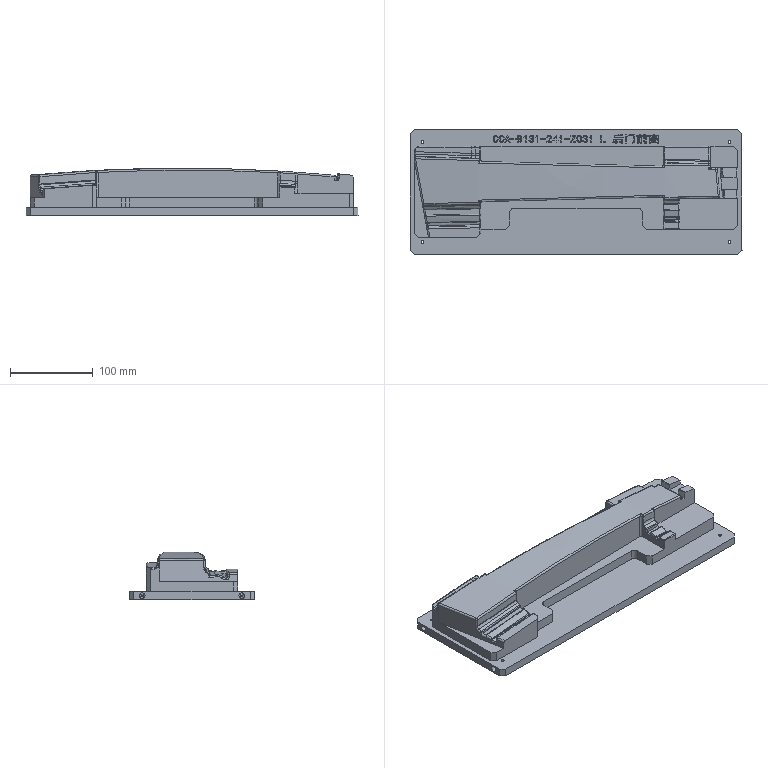NC program | NX | posted with a generic post | part box 400 x 150 x 57.494 mm
Lines 6500 to 7057 of 7057:
(A5 , TOOL : D10)
N12980 M6
N12982 G54
N12984 G17 G0 G90 X-193. Y-85.002 S3500 M3
N12986 G43 Z20.002 H0
N12988 Z9.802
N12990 G94 G1 Z9.502 F2000.
N12992 Y-82.002
N12994 G3 X-195. Y-80.002 R2.
N12996 G2 X-198.536 Y-78.538 R5.
N12998 G1 X-203.536 Y-73.538
N13000 G2 X-205. Y-70.002 R5.
N13002 G1 Y69.998
N13004 G2 X-203.536 Y73.533 R5.
N13006 G1 X-198.536 Y78.533
N13008 G2 X-195. Y79.998 R5.
N13010 G1 X195. Z9.503
N13012 G2 X198.536 Y78.533 R5.
N13014 G1 X203.536 Y73.533
N13016 G2 X205. Y69.998 R5.
N13018 G1 Y-70.002
N13020 G2 X203.536 Y-73.538 R5.
N13022 G1 X198.536 Y-78.538
N13024 G2 X195. Y-80.002 R5.
N13026 G1 X-195. Z9.502
N13028 G3 X-197. Y-82.002 R2.
N13030 G1 Y-84.8
N13032 Z9.802
N13034 G0 Z10.302
N13036 X-193. Y-85.002
N13038 Z9.302
N13040 G1 Z9.002
N13042 Y-82.002
N13044 G3 X-195. Y-80.002 R2.
N13046 G2 X-198.536 Y-78.538 R5.
N13048 G1 X-203.536 Y-73.538
N13050 G2 X-205. Y-70.002 R5.
N13052 G1 Y69.998
N13054 G2 X-203.536 Y73.533 R5.
N13056 G1 X-198.536 Y78.533
N13058 G2 X-195. Y79.998 R5.
N13060 G1 X195. Z9.003
N13062 G2 X198.536 Y78.533 R5.
N13064 G1 X203.536 Y73.533
N13066 G2 X205. Y69.998 R5.
N13068 G1 Y-70.002
N13070 G2 X203.536 Y-73.538 R5.
N13072 G1 X198.536 Y-78.538
N13074 G2 X195. Y-80.002 R5.
N13076 G1 X-195. Z9.002
N13078 G3 X-197. Y-82.002 R2.
N13080 G1 Y-84.8
N13082 Z9.302
N13084 G0 Z9.802
N13086 X-193. Y-85.002
N13088 Z8.802
N13090 G1 Z8.502
N13092 Y-82.002
N13094 G3 X-195. Y-80.002 R2.
N13096 G2 X-198.536 Y-78.538 R5.
N13098 G1 X-203.536 Y-73.538
N13100 G2 X-205. Y-70.002 R5.
N13102 G1 Y69.998
N13104 G2 X-203.536 Y73.533 R5.
N13106 G1 X-198.536 Y78.533
N13108 G2 X-195. Y79.998 R5.
N13110 G1 X195. Z8.503
N13112 G2 X198.536 Y78.533 R5.
N13114 G1 X203.536 Y73.533
N13116 G2 X205. Y69.998 R5.
N13118 G1 Y-70.002
N13120 G2 X203.536 Y-73.538 R5.
N13122 G1 X198.536 Y-78.538
N13124 G2 X195. Y-80.002 R5.
N13126 G1 X-195. Z8.502
N13128 G3 X-197. Y-82.002 R2.
N13130 G1 Y-84.8
N13132 Z8.802
N13134 G0 Z9.302
N13136 X-193. Y-85.002
N13138 Z8.302
N13140 G1 Z8.002
N13142 Y-82.002
N13144 G3 X-195. Y-80.002 R2.
N13146 G2 X-198.536 Y-78.538 R5.
N13148 G1 X-203.536 Y-73.538
N13150 G2 X-205. Y-70.002 R5.
N13152 G1 Y69.998
N13154 G2 X-203.536 Y73.533 R5.
N13156 G1 X-198.536 Y78.533
N13158 G2 X-195. Y79.998 R5.
N13160 G1 X195. Z8.003
N13162 G2 X198.536 Y78.533 R5.
N13164 G1 X203.536 Y73.533
N13166 G2 X205. Y69.998 R5.
N13168 G1 Y-70.002
N13170 G2 X203.536 Y-73.538 R5.
N13172 G1 X198.536 Y-78.538
N13174 G2 X195. Y-80.002 R5.
N13176 G1 X-195. Z8.002
N13178 G3 X-197. Y-82.002 R2.
N13180 G1 Y-84.8
N13182 Z8.302
N13184 G0 Z8.802
N13186 X-193. Y-85.002
N13188 Z7.802
N13190 G1 Z7.502
N13192 Y-82.002
N13194 G3 X-195. Y-80.002 R2.
N13196 G2 X-198.536 Y-78.538 R5.
N13198 G1 X-203.536 Y-73.538
N13200 G2 X-205. Y-70.002 R5.
N13202 G1 Y69.998
N13204 G2 X-203.536 Y73.533 R5.
N13206 G1 X-198.536 Y78.533
N13208 G2 X-195. Y79.998 R5.
N13210 G1 X195. Z7.503
N13212 G2 X198.536 Y78.533 R5.
N13214 G1 X203.536 Y73.533
N13216 G2 X205. Y69.998 R5.
N13218 G1 Y-70.002
N13220 G2 X203.536 Y-73.538 R5.
N13222 G1 X198.536 Y-78.538
N13224 G2 X195. Y-80.002 R5.
N13226 G1 X-195. Z7.502
N13228 G3 X-197. Y-82.002 R2.
N13230 G1 Y-84.8
N13232 Z7.802
N13234 G0 Z8.302
N13236 X-193. Y-85.002
N13238 Z7.302
N13240 G1 Z7.002
N13242 Y-82.002
N13244 G3 X-195. Y-80.002 R2.
N13246 G2 X-198.536 Y-78.538 R5.
N13248 G1 X-203.536 Y-73.538
N13250 G2 X-205. Y-70.002 R5.
N13252 G1 Y69.998
N13254 G2 X-203.536 Y73.533 R5.
N13256 G1 X-198.536 Y78.533
N13258 G2 X-195. Y79.998 R5.
N13260 G1 X195. Z7.003
N13262 G2 X198.536 Y78.533 R5.
N13264 G1 X203.536 Y73.533
N13266 G2 X205. Y69.998 R5.
N13268 G1 Y-70.002
N13270 G2 X203.536 Y-73.538 R5.
N13272 G1 X198.536 Y-78.538
N13274 G2 X195. Y-80.002 R5.
N13276 G1 X-195. Z7.002
N13278 G3 X-197. Y-82.002 R2.
N13280 G1 Y-84.8
N13282 Z7.302
N13284 G0 Z7.802
N13286 X-193. Y-85.002
N13288 Z6.802
N13290 G1 Z6.502
N13292 Y-82.002
N13294 G3 X-195. Y-80.002 R2.
N13296 G2 X-198.536 Y-78.538 R5.
N13298 G1 X-203.536 Y-73.538
N13300 G2 X-205. Y-70.002 R5.
N13302 G1 Y69.998
N13304 G2 X-203.536 Y73.533 R5.
N13306 G1 X-198.536 Y78.533
N13308 G2 X-195. Y79.998 R5.
N13310 G1 X195. Z6.503
N13312 G2 X198.536 Y78.533 R5.
N13314 G1 X203.536 Y73.533
N13316 G2 X205. Y69.998 R5.
N13318 G1 Y-70.002
N13320 G2 X203.536 Y-73.538 R5.
N13322 G1 X198.536 Y-78.538
N13324 G2 X195. Y-80.002 R5.
N13326 G1 X-195. Z6.502
N13328 G3 X-197. Y-82.002 R2.
N13330 G1 Y-84.8
N13332 Z6.802
N13334 G0 Z7.302
N13336 X-193. Y-85.002
N13338 Z6.302
N13340 G1 Z6.002
N13342 Y-82.002
N13344 G3 X-195. Y-80.002 R2.
N13346 G2 X-198.536 Y-78.538 R5.
N13348 G1 X-203.536 Y-73.538
N13350 G2 X-205. Y-70.002 R5.
N13352 G1 Y69.998
N13354 G2 X-203.536 Y73.533 R5.
N13356 G1 X-198.536 Y78.533
N13358 G2 X-195. Y79.998 R5.
N13360 G1 X195. Z6.003
N13362 G2 X198.536 Y78.533 R5.
N13364 G1 X203.536 Y73.533
N13366 G2 X205. Y69.998 R5.
N13368 G1 Y-70.002
N13370 G2 X203.536 Y-73.538 R5.
N13372 G1 X198.536 Y-78.538
N13374 G2 X195. Y-80.002 R5.
N13376 G1 X-195. Z6.002
N13378 G3 X-197. Y-82.002 R2.
N13380 G1 Y-84.8
N13382 Z6.302
N13384 G0 Z6.802
N13386 X-193. Y-85.002
N13388 Z5.802
N13390 G1 Z5.502
N13392 Y-82.002
N13394 G3 X-195. Y-80.002 R2.
N13396 G2 X-198.536 Y-78.538 R5.
N13398 G1 X-203.536 Y-73.538
N13400 G2 X-205. Y-70.002 R5.
N13402 G1 Y69.998
N13404 G2 X-203.536 Y73.533 R5.
N13406 G1 X-198.536 Y78.533
N13408 G2 X-195. Y79.998 R5.
N13410 G1 X195. Z5.503
N13412 G2 X198.536 Y78.533 R5.
N13414 G1 X203.536 Y73.533
N13416 G2 X205. Y69.998 R5.
N13418 G1 Y-70.002
N13420 G2 X203.536 Y-73.538 R5.
N13422 G1 X198.536 Y-78.538
N13424 G2 X195. Y-80.002 R5.
N13426 G1 X-195. Z5.502
N13428 G3 X-197. Y-82.002 R2.
N13430 G1 Y-84.8
N13432 Z5.802
N13434 G0 Z6.302
N13436 X-193. Y-85.002
N13438 Z5.302
N13440 G1 Z5.002
N13442 Y-82.002
N13444 G3 X-195. Y-80.002 R2.
N13446 G2 X-198.536 Y-78.538 R5.
N13448 G1 X-203.536 Y-73.538
N13450 G2 X-205. Y-70.002 R5.
N13452 G1 Y69.998
N13454 G2 X-203.536 Y73.533 R5.
N13456 G1 X-198.536 Y78.533
N13458 G2 X-195. Y79.998 R5.
N13460 G1 X195. Z5.003
N13462 G2 X198.536 Y78.533 R5.
N13464 G1 X203.536 Y73.533
N13466 G2 X205. Y69.998 R5.
N13468 G1 Y-70.002
N13470 G2 X203.536 Y-73.538 R5.
N13472 G1 X198.536 Y-78.538
N13474 G2 X195. Y-80.002 R5.
N13476 G1 X-195. Z5.002
N13478 G3 X-197. Y-82.002 R2.
N13480 G1 Y-84.8
N13482 Z5.302
N13484 G0 Z5.802
N13486 X-193. Y-85.002
N13488 Z4.802
N13490 G1 Z4.502
N13492 Y-82.002
N13494 G3 X-195. Y-80.002 R2.
N13496 G2 X-198.536 Y-78.538 R5.
N13498 G1 X-203.536 Y-73.538
N13500 G2 X-205. Y-70.002 R5.
N13502 G1 Y69.998
N13504 G2 X-203.536 Y73.533 R5.
N13506 G1 X-198.536 Y78.533
N13508 G2 X-195. Y79.998 R5.
N13510 G1 X195. Z4.503
N13512 G2 X198.536 Y78.533 R5.
N13514 G1 X203.536 Y73.533
N13516 G2 X205. Y69.998 R5.
N13518 G1 Y-70.002
N13520 G2 X203.536 Y-73.538 R5.
N13522 G1 X198.536 Y-78.538
N13524 G2 X195. Y-80.002 R5.
N13526 G1 X-195. Z4.502
N13528 G3 X-197. Y-82.002 R2.
N13530 G1 Y-84.8
N13532 Z4.802
N13534 G0 Z5.302
N13536 X-193. Y-85.002
N13538 Z4.302
N13540 G1 Z4.002
N13542 Y-82.002
N13544 G3 X-195. Y-80.002 R2.
N13546 G2 X-198.536 Y-78.538 R5.
N13548 G1 X-203.536 Y-73.538
N13550 G2 X-205. Y-70.002 R5.
N13552 G1 Y69.998
N13554 G2 X-203.536 Y73.533 R5.
N13556 G1 X-198.536 Y78.533
N13558 G2 X-195. Y79.998 R5.
N13560 G1 X195. Z4.003
N13562 G2 X198.536 Y78.533 R5.
N13564 G1 X203.536 Y73.533
N13566 G2 X205. Y69.998 R5.
N13568 G1 Y-70.002
N13570 G2 X203.536 Y-73.538 R5.
N13572 G1 X198.536 Y-78.538
N13574 G2 X195. Y-80.002 R5.
N13576 G1 X-195. Z4.002
N13578 G3 X-197. Y-82.002 R2.
N13580 G1 Y-84.8
N13582 Z4.302
N13584 G0 Z4.802
N13586 X-193. Y-85.002
N13588 Z3.802
N13590 G1 Z3.502
N13592 Y-82.002
N13594 G3 X-195. Y-80.002 R2.
N13596 G2 X-198.536 Y-78.538 R5.
N13598 G1 X-203.536 Y-73.538
N13600 G2 X-205. Y-70.002 R5.
N13602 G1 Y69.998
N13604 G2 X-203.536 Y73.533 R5.
N13606 G1 X-198.536 Y78.533
N13608 G2 X-195. Y79.998 R5.
N13610 G1 X195. Z3.503
N13612 G2 X198.536 Y78.533 R5.
N13614 G1 X203.536 Y73.533
N13616 G2 X205. Y69.998 R5.
N13618 G1 Y-70.002
N13620 G2 X203.536 Y-73.538 R5.
N13622 G1 X198.536 Y-78.538
N13624 G2 X195. Y-80.002 R5.
N13626 G1 X-195. Z3.502
N13628 G3 X-197. Y-82.002 R2.
N13630 G1 Y-84.8
N13632 Z3.802
N13634 G0 Z4.302
N13636 X-193. Y-85.002
N13638 Z3.302
N13640 G1 Z3.002
N13642 Y-82.002
N13644 G3 X-195. Y-80.002 R2.
N13646 G2 X-198.536 Y-78.538 R5.
N13648 G1 X-203.536 Y-73.538
N13650 G2 X-205. Y-70.002 R5.
N13652 G1 Y69.998
N13654 G2 X-203.536 Y73.533 R5.
N13656 G1 X-198.536 Y78.533
N13658 G2 X-195. Y79.998 R5.
N13660 G1 X195. Z3.003
N13662 G2 X198.536 Y78.533 R5.
N13664 G1 X203.536 Y73.533
N13666 G2 X205. Y69.998 R5.
N13668 G1 Y-70.002
N13670 G2 X203.536 Y-73.538 R5.
N13672 G1 X198.536 Y-78.538
N13674 G2 X195. Y-80.002 R5.
N13676 G1 X-195. Z3.002
N13678 G3 X-197. Y-82.002 R2.
N13680 G1 Y-84.8
N13682 Z3.302
N13684 G0 Z3.802
N13686 X-193. Y-85.002
N13688 Z2.802
N13690 G1 Z2.502
N13692 Y-82.002
N13694 G3 X-195. Y-80.002 R2.
N13696 G2 X-198.536 Y-78.538 R5.
N13698 G1 X-203.536 Y-73.538
N13700 G2 X-205. Y-70.002 R5.
N13702 G1 Y69.998
N13704 G2 X-203.536 Y73.533 R5.
N13706 G1 X-198.536 Y78.533
N13708 G2 X-195. Y79.998 R5.
N13710 G1 X195. Z2.503
N13712 G2 X198.536 Y78.533 R5.
N13714 G1 X203.536 Y73.533
N13716 G2 X205. Y69.998 R5.
N13718 G1 Y-70.002
N13720 G2 X203.536 Y-73.538 R5.
N13722 G1 X198.536 Y-78.538
N13724 G2 X195. Y-80.002 R5.
N13726 G1 X-195. Z2.502
N13728 G3 X-197. Y-82.002 R2.
N13730 G1 Y-84.8
N13732 Z2.802
N13734 G0 Z3.302
N13736 X-193. Y-85.002
N13738 Z2.302
N13740 G1 Z2.002
N13742 Y-82.002
N13744 G3 X-195. Y-80.002 R2.
N13746 G2 X-198.536 Y-78.538 R5.
N13748 G1 X-203.536 Y-73.538
N13750 G2 X-205. Y-70.002 R5.
N13752 G1 Y69.998
N13754 G2 X-203.536 Y73.533 R5.
N13756 G1 X-198.536 Y78.533
N13758 G2 X-195. Y79.998 R5.
N13760 G1 X195. Z2.003
N13762 G2 X198.536 Y78.533 R5.
N13764 G1 X203.536 Y73.533
N13766 G2 X205. Y69.998 R5.
N13768 G1 Y-70.002
N13770 G2 X203.536 Y-73.538 R5.
N13772 G1 X198.536 Y-78.538
N13774 G2 X195. Y-80.002 R5.
N13776 G1 X-195. Z2.002
N13778 G3 X-197. Y-82.002 R2.
N13780 G1 Y-84.8
N13782 Z2.302
N13784 G0 Z2.802
N13786 X-193. Y-85.002
N13788 Z1.802
N13790 G1 Z1.502
N13792 Y-82.002
N13794 G3 X-195. Y-80.002 R2.
N13796 G2 X-198.536 Y-78.538 R5.
N13798 G1 X-203.536 Y-73.538
N13800 G2 X-205. Y-70.002 R5.
N13802 G1 Y69.998
N13804 G2 X-203.536 Y73.533 R5.
N13806 G1 X-198.536 Y78.533
N13808 G2 X-195. Y79.998 R5.
N13810 G1 X195. Z1.503
N13812 G2 X198.536 Y78.533 R5.
N13814 G1 X203.536 Y73.533
N13816 G2 X205. Y69.998 R5.
N13818 G1 Y-70.002
N13820 G2 X203.536 Y-73.538 R5.
N13822 G1 X198.536 Y-78.538
N13824 G2 X195. Y-80.002 R5.
N13826 G1 X-195. Z1.502
N13828 G3 X-197. Y-82.002 R2.
N13830 G1 Y-84.8
N13832 Z1.802
N13834 G0 Z2.302
N13836 X-193. Y-85.002
N13838 Z1.302
N13840 G1 Z1.002
N13842 Y-82.002
N13844 G3 X-195. Y-80.002 R2.
N13846 G2 X-198.536 Y-78.538 R5.
N13848 G1 X-203.536 Y-73.538
N13850 G2 X-205. Y-70.002 R5.
N13852 G1 Y69.998
N13854 G2 X-203.536 Y73.533 R5.
N13856 G1 X-198.536 Y78.533
N13858 G2 X-195. Y79.998 R5.
N13860 G1 X195. Z1.003
N13862 G2 X198.536 Y78.533 R5.
N13864 G1 X203.536 Y73.533
N13866 G2 X205. Y69.998 R5.
N13868 G1 Y-70.002
N13870 G2 X203.536 Y-73.538 R5.
N13872 G1 X198.536 Y-78.538
N13874 G2 X195. Y-80.002 R5.
N13876 G1 X-195. Z1.002
N13878 G3 X-197. Y-82.002 R2.
N13880 G1 Y-84.8
N13882 Z1.302
N13884 G0 Z1.802
N13886 X-193. Y-85.002
N13888 Z0.802
N13890 G1 Z0.502
N13892 Y-82.002
N13894 G3 X-195. Y-80.002 R2.
N13896 G2 X-198.536 Y-78.538 R5.
N13898 G1 X-203.536 Y-73.538
N13900 G2 X-205. Y-70.002 R5.
N13902 G1 Y69.998
N13904 G2 X-203.536 Y73.533 R5.
N13906 G1 X-198.536 Y78.533
N13908 G2 X-195. Y79.998 R5.
N13910 G1 X195. Z0.503
N13912 G2 X198.536 Y78.533 R5.
N13914 G1 X203.536 Y73.533
N13916 G2 X205. Y69.998 R5.
N13918 G1 Y-70.002
N13920 G2 X203.536 Y-73.538 R5.
N13922 G1 X198.536 Y-78.538
N13924 G2 X195. Y-80.002 R5.
N13926 G1 X-195. Z0.502
N13928 G3 X-197. Y-82.002 R2.
N13930 G1 Y-84.8
N13932 Z0.802
N13934 G0 Z1.302
N13936 X-193. Y-85.002
N13938 Z0.302
N13940 G1 Z0.002
N13942 Y-82.002
N13944 G3 X-195. Y-80.002 R2.
N13946 G2 X-198.536 Y-78.538 R5.
N13948 G1 X-203.536 Y-73.538
N13950 G2 X-205. Y-70.002 R5.
N13952 G1 Y69.998
N13954 G2 X-203.536 Y73.533 R5.
N13956 G1 X-198.536 Y78.533
N13958 G2 X-195. Y79.998 R5.
N13960 G1 X195. Z0.003
N13962 G2 X198.536 Y78.533 R5.
N13964 G1 X203.536 Y73.533
N13966 G2 X205. Y69.998 R5.
N13968 G1 Y-70.002
N13970 G2 X203.536 Y-73.538 R5.
N13972 G1 X198.536 Y-78.538
N13974 G2 X195. Y-80.002 R5.
N13976 G1 X-195. Z0.002
N13978 G3 X-197. Y-82.002 R2.
N13980 G1 Y-84.8
N13982 Z0.302
N13984 G0 Z0.802
N13986 X-193. Y-85.002
N13988 Z-0.198
N13990 G1 Z-0.498
N13992 Y-82.002
N13994 G3 X-195. Y-80.002 R2.
N13996 G2 X-198.536 Y-78.538 R5.
N13998 G1 X-203.536 Y-73.538
N14000 G2 X-205. Y-70.002 R5.
N14002 G1 Y69.998
N14004 G2 X-203.536 Y73.533 R5.
N14006 G1 X-198.536 Y78.533
N14008 G2 X-195. Y79.998 R5.
N14010 G1 X195. Z-0.497
N14012 G2 X198.536 Y78.533 R5.
N14014 G1 X203.536 Y73.533
N14016 G2 X205. Y69.998 R5.
N14018 G1 Y-70.002
N14020 G2 X203.536 Y-73.538 R5.
N14022 G1 X198.536 Y-78.538
N14024 G2 X195. Y-80.002 R5.
N14026 G1 X-195. Z-0.498
N14028 G3 X-197. Y-82.002 R2.
N14030 G1 Y-84.8
N14032 Z-0.198
N14034 G0 Z0.302
N14036 X-193. Y-85.002
N14038 Z-0.698
N14040 G1 Z-0.998
N14042 Y-82.002
N14044 G3 X-195. Y-80.002 R2.
N14046 G2 X-198.536 Y-78.538 R5.
N14048 G1 X-203.536 Y-73.538
N14050 G2 X-205. Y-70.002 R5.
N14052 G1 Y69.998
N14054 G2 X-203.536 Y73.533 R5.
N14056 G1 X-198.536 Y78.533
N14058 G2 X-195. Y79.998 R5.
N14060 G1 X195. Z-0.997
N14062 G2 X198.536 Y78.533 R5.
N14064 G1 X203.536 Y73.533
N14066 G2 X205. Y69.998 R5.
N14068 G1 Y-70.002
N14070 G2 X203.536 Y-73.538 R5.
N14072 G1 X198.536 Y-78.538
N14074 G2 X195. Y-80.002 R5.
N14076 G1 X-195. Z-0.998
N14078 G3 X-197. Y-82.002 R2.
N14080 G1 Y-84.8
N14082 Z-0.698
N14084 G0 Z20.002
N14086 M5
N14088 M2